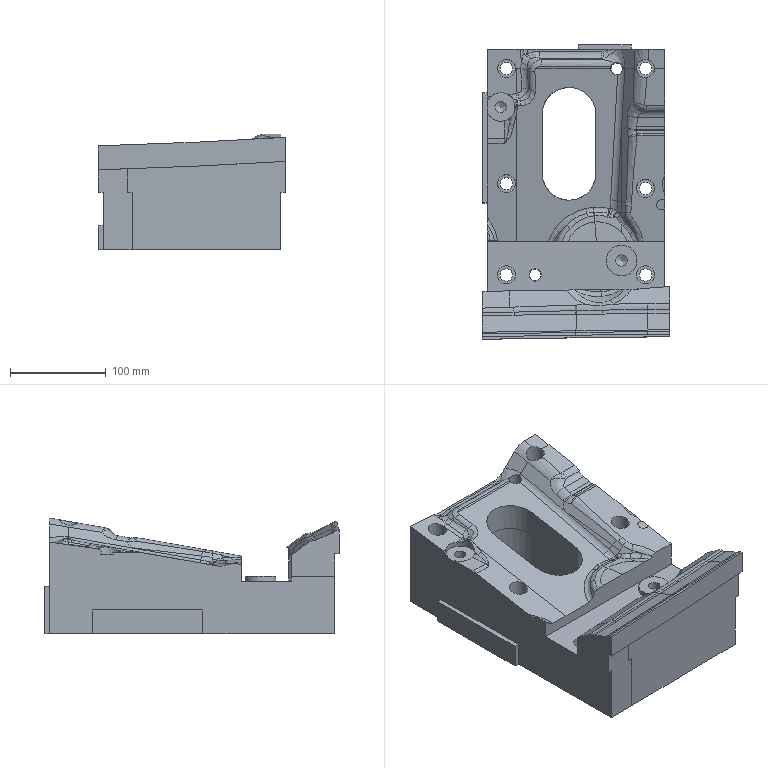Part | NX | features solid 2 | 1 solid | 226 faces | box 195 x 307.268 x 120.895 mm | volume 3919488 mm3 | spline 123 | cylinder 51 | plane 48 | cone 3 | sphere 1 | commonest cylinder face diameters 20 x9 13 x8 19 x6 12 x4 16 x4 20.001 x4